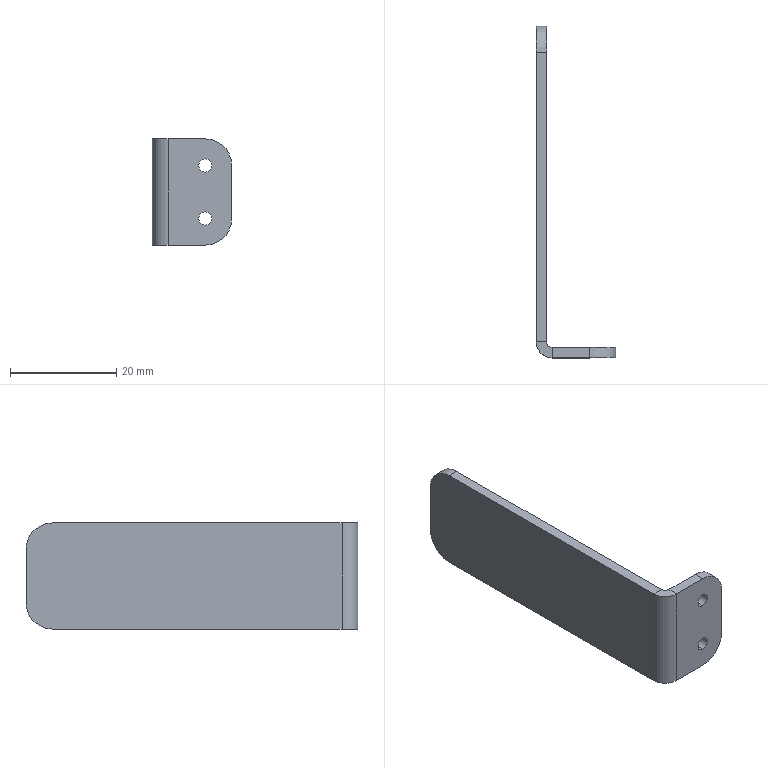Part | SolidWorks | features BreakCorner 1, FlatPattern 1, HoleWzd 1, SMBaseFlange 1, SheetMetal 1 | 1 solid | 22 faces | box 15 x 62.5 x 20 mm | volume 2923 mm3 | plane 12 | cylinder 10 | commonest cylinder face diameters 2.5 x4 10 x4 2 x1 6 x1
STEP:
#1=CARTESIAN_POINT('',(10.,0.,-6.25));
#2=VERTEX_POINT('',#1);
#3=CARTESIAN_POINT('',(10.,0.,-3.75));
#4=VERTEX_POINT('',#3);
#5=CARTESIAN_POINT('',(10.,0.,-5.));
#6=DIRECTION('',(0.,1.,0.));
#7=DIRECTION('',(0.,0.,1.));
#8=AXIS2_PLACEMENT_3D('',#5,#6,#7);
#9=CIRCLE('',#8,1.25);
#10=EDGE_CURVE('',#2,#4,#9,.T.);
#11=ORIENTED_EDGE('',*,*,#10,.F.);
#12=CARTESIAN_POINT('',(10.,2.,-6.25));
#13=VERTEX_POINT('',#12);
#14=CARTESIAN_POINT('',(10.,2.,-6.25));
#15=DIRECTION('',(0.,1.,0.));
#16=VECTOR('',#15,1000.);
#17=LINE('',#14,#16);
#18=EDGE_CURVE('',#2,#13,#17,.T.);
#19=ORIENTED_EDGE('',*,*,#18,.T.);
#20=CARTESIAN_POINT('',(10.,2.,-3.75));
#21=VERTEX_POINT('',#20);
#22=CARTESIAN_POINT('',(10.,2.,-5.));
#23=DIRECTION('',(0.,1.,0.));
#24=DIRECTION('',(0.,0.,1.));
#25=AXIS2_PLACEMENT_3D('',#22,#23,#24);
#26=CIRCLE('',#25,1.25);
#27=EDGE_CURVE('',#13,#21,#26,.T.);
#28=ORIENTED_EDGE('',*,*,#27,.T.);
#29=CARTESIAN_POINT('',(10.,2.,-3.75));
#30=DIRECTION('',(0.,1.,0.));
#31=VECTOR('',#30,1000.);
#32=LINE('',#29,#31);
#33=EDGE_CURVE('',#4,#21,#32,.T.);
#34=ORIENTED_EDGE('',*,*,#33,.F.);
#35=EDGE_LOOP('',(#11,#19,#28,#34));
#36=FACE_OUTER_BOUND('',#35,.T.);
#37=CARTESIAN_POINT('',(10.,2.,-5.));
#38=DIRECTION('',(0.,1.,0.));
#39=DIRECTION('',(0.,0.,1.));
#40=AXIS2_PLACEMENT_3D('',#37,#38,#39);
#41=CYLINDRICAL_SURFACE('',#40,1.25);
#42=ADVANCED_FACE('',(#36),#41,.F.);
#43=CARTESIAN_POINT('',(10.,0.,3.75));
#44=VERTEX_POINT('',#43);
#45=CARTESIAN_POINT('',(10.,0.,6.25));
#46=VERTEX_POINT('',#45);
#47=CARTESIAN_POINT('',(10.,0.,5.));
#48=DIRECTION('',(0.,1.,0.));
#49=DIRECTION('',(0.,0.,1.));
#50=AXIS2_PLACEMENT_3D('',#47,#48,#49);
#51=CIRCLE('',#50,1.25);
#52=EDGE_CURVE('',#44,#46,#51,.T.);
#53=ORIENTED_EDGE('',*,*,#52,.F.);
#54=CARTESIAN_POINT('',(10.,2.,3.75));
#55=VERTEX_POINT('',#54);
#56=CARTESIAN_POINT('',(10.,2.,3.75));
#57=DIRECTION('',(0.,1.,0.));
#58=VECTOR('',#57,1000.);
#59=LINE('',#56,#58);
#60=EDGE_CURVE('',#44,#55,#59,.T.);
#61=ORIENTED_EDGE('',*,*,#60,.T.);
#62=CARTESIAN_POINT('',(10.,2.,6.25));
#63=VERTEX_POINT('',#62);
#64=CARTESIAN_POINT('',(10.,2.,5.));
#65=DIRECTION('',(0.,1.,0.));
#66=DIRECTION('',(0.,0.,1.));
#67=AXIS2_PLACEMENT_3D('',#64,#65,#66);
#68=CIRCLE('',#67,1.25);
#69=EDGE_CURVE('',#55,#63,#68,.T.);
#70=ORIENTED_EDGE('',*,*,#69,.T.);
#71=CARTESIAN_POINT('',(10.,2.,6.25));
#72=DIRECTION('',(0.,1.,0.));
#73=VECTOR('',#72,1000.);
#74=LINE('',#71,#73);
#75=EDGE_CURVE('',#46,#63,#74,.T.);
#76=ORIENTED_EDGE('',*,*,#75,.F.);
#77=EDGE_LOOP('',(#53,#61,#70,#76));
#78=FACE_OUTER_BOUND('',#77,.T.);
#79=CARTESIAN_POINT('',(10.,2.,5.));
#80=DIRECTION('',(0.,1.,0.));
#81=DIRECTION('',(0.,0.,1.));
#82=AXIS2_PLACEMENT_3D('',#79,#80,#81);
#83=CYLINDRICAL_SURFACE('',#82,1.25);
#84=ADVANCED_FACE('',(#78),#83,.F.);
#85=CARTESIAN_POINT('',(0.,3.,10.));
#86=VERTEX_POINT('',#85);
#87=CARTESIAN_POINT('',(2.,3.,10.));
#88=VERTEX_POINT('',#87);
#89=CARTESIAN_POINT('',(0.,3.,10.));
#90=DIRECTION('',(1.,0.,0.));
#91=VECTOR('',#90,1000.);
#92=LINE('',#89,#91);
#93=EDGE_CURVE('',#86,#88,#92,.T.);
#94=ORIENTED_EDGE('',*,*,#93,.F.);
#95=CARTESIAN_POINT('',(3.,0.,10.));
#96=VERTEX_POINT('',#95);
#97=CARTESIAN_POINT('',(3.,3.,10.));
#98=DIRECTION('',(0.,0.,1.));
#99=DIRECTION('',(-1.,0.,0.));
#100=AXIS2_PLACEMENT_3D('',#97,#98,#99);
#101=CIRCLE('',#100,3.);
#102=EDGE_CURVE('',#86,#96,#101,.T.);
#103=ORIENTED_EDGE('',*,*,#102,.T.);
#104=CARTESIAN_POINT('',(3.,2.,10.));
#105=VERTEX_POINT('',#104);
#106=CARTESIAN_POINT('',(3.,2.,10.));
#107=DIRECTION('',(0.,-1.,0.));
#108=VECTOR('',#107,1000.);
#109=LINE('',#106,#108);
#110=EDGE_CURVE('',#105,#96,#109,.T.);
#111=ORIENTED_EDGE('',*,*,#110,.F.);
#112=CARTESIAN_POINT('',(3.,3.,10.));
#113=DIRECTION('',(0.,0.,1.));
#114=DIRECTION('',(1.,0.,0.));
#115=AXIS2_PLACEMENT_3D('',#112,#113,#114);
#116=CIRCLE('',#115,1.);
#117=EDGE_CURVE('',#88,#105,#116,.T.);
#118=ORIENTED_EDGE('',*,*,#117,.F.);
#119=EDGE_LOOP('',(#94,#103,#111,#118));
#120=FACE_OUTER_BOUND('',#119,.T.);
#121=CARTESIAN_POINT('',(0.,3.,10.));
#122=DIRECTION('',(0.,0.,1.));
#123=DIRECTION('',(1.,0.,0.));
#124=AXIS2_PLACEMENT_3D('',#121,#122,#123);
#125=PLANE('',#124);
#126=ADVANCED_FACE('',(#120),#125,.T.);
#127=CARTESIAN_POINT('',(2.,57.5,10.));
#128=VERTEX_POINT('',#127);
#129=CARTESIAN_POINT('',(2.,62.5,10.));
#130=DIRECTION('',(0.,-1.,0.));
#131=VECTOR('',#130,1000.);
#132=LINE('',#129,#131);
#133=EDGE_CURVE('',#128,#88,#132,.T.);
#134=ORIENTED_EDGE('',*,*,#133,.F.);
#135=CARTESIAN_POINT('',(0.,57.5,10.));
#136=VERTEX_POINT('',#135);
#137=CARTESIAN_POINT('',(3.,57.5,10.));
#138=DIRECTION('',(-1.,0.,0.));
#139=VECTOR('',#138,1000.);
#140=LINE('',#137,#139);
#141=EDGE_CURVE('',#128,#136,#140,.T.);
#142=ORIENTED_EDGE('',*,*,#141,.T.);
#143=CARTESIAN_POINT('',(0.,62.5,10.));
#144=DIRECTION('',(0.,-1.,0.));
#145=VECTOR('',#144,1000.);
#146=LINE('',#143,#145);
#147=EDGE_CURVE('',#136,#86,#146,.T.);
#148=ORIENTED_EDGE('',*,*,#147,.T.);
#149=ORIENTED_EDGE('',*,*,#93,.T.);
#150=EDGE_LOOP('',(#134,#142,#148,#149));
#151=FACE_OUTER_BOUND('',#150,.T.);
#152=CARTESIAN_POINT('',(3.,2.,10.));
#153=DIRECTION('',(0.,0.,1.));
#154=DIRECTION('',(1.,0.,0.));
#155=AXIS2_PLACEMENT_3D('',#152,#153,#154);
#156=PLANE('',#155);
#157=ADVANCED_FACE('',(#151),#156,.T.);
#158=CARTESIAN_POINT('',(3.,0.,-10.));
#159=VERTEX_POINT('',#158);
#160=CARTESIAN_POINT('',(3.,2.,-10.));
#161=VERTEX_POINT('',#160);
#162=CARTESIAN_POINT('',(3.,0.,-10.));
#163=DIRECTION('',(0.,1.,0.));
#164=VECTOR('',#163,1000.);
#165=LINE('',#162,#164);
#166=EDGE_CURVE('',#159,#161,#165,.T.);
#167=ORIENTED_EDGE('',*,*,#166,.F.);
#168=CARTESIAN_POINT('',(0.,3.,-10.));
#169=VERTEX_POINT('',#168);
#170=CARTESIAN_POINT('',(3.,3.,-10.));
#171=DIRECTION('',(0.,0.,1.));
#172=DIRECTION('',(-1.,0.,0.));
#173=AXIS2_PLACEMENT_3D('',#170,#171,#172);
#174=CIRCLE('',#173,3.);
#175=EDGE_CURVE('',#169,#159,#174,.T.);
#176=ORIENTED_EDGE('',*,*,#175,.F.);
#177=CARTESIAN_POINT('',(2.,3.,-10.));
#178=VERTEX_POINT('',#177);
#179=CARTESIAN_POINT('',(2.,3.,-10.));
#180=DIRECTION('',(-1.,0.,0.));
#181=VECTOR('',#180,1000.);
#182=LINE('',#179,#181);
#183=EDGE_CURVE('',#178,#169,#182,.T.);
#184=ORIENTED_EDGE('',*,*,#183,.F.);
#185=CARTESIAN_POINT('',(3.,3.,-10.));
#186=DIRECTION('',(0.,0.,1.));
#187=DIRECTION('',(1.,0.,0.));
#188=AXIS2_PLACEMENT_3D('',#185,#186,#187);
#189=CIRCLE('',#188,1.);
#190=EDGE_CURVE('',#178,#161,#189,.T.);
#191=ORIENTED_EDGE('',*,*,#190,.T.);
#192=EDGE_LOOP('',(#167,#176,#184,#191));
#193=FACE_OUTER_BOUND('',#192,.T.);
#194=CARTESIAN_POINT('',(3.,0.,-10.));
#195=DIRECTION('',(0.,0.,-1.));
#196=DIRECTION('',(-1.,0.,0.));
#197=AXIS2_PLACEMENT_3D('',#194,#195,#196);
#198=PLANE('',#197);
#199=ADVANCED_FACE('',(#193),#198,.T.);
#200=CARTESIAN_POINT('',(10.,2.,-10.));
#201=VERTEX_POINT('',#200);
#202=CARTESIAN_POINT('',(0.,2.,-10.));
#203=DIRECTION('',(1.,0.,0.));
#204=VECTOR('',#203,1000.);
#205=LINE('',#202,#204);
#206=EDGE_CURVE('',#161,#201,#205,.T.);
#207=ORIENTED_EDGE('',*,*,#206,.T.);
#208=CARTESIAN_POINT('',(10.,0.,-10.));
#209=VERTEX_POINT('',#208);
#210=CARTESIAN_POINT('',(10.,3.,-10.));
#211=DIRECTION('',(0.,-1.,0.));
#212=VECTOR('',#211,1000.);
#213=LINE('',#210,#212);
#214=EDGE_CURVE('',#201,#209,#213,.T.);
#215=ORIENTED_EDGE('',*,*,#214,.T.);
#216=CARTESIAN_POINT('',(0.,0.,-10.));
#217=DIRECTION('',(1.,0.,0.));
#218=VECTOR('',#217,1000.);
#219=LINE('',#216,#218);
#220=EDGE_CURVE('',#159,#209,#219,.T.);
#221=ORIENTED_EDGE('',*,*,#220,.F.);
#222=ORIENTED_EDGE('',*,*,#166,.T.);
#223=EDGE_LOOP('',(#207,#215,#221,#222));
#224=FACE_OUTER_BOUND('',#223,.T.);
#225=CARTESIAN_POINT('',(2.,3.,-10.));
#226=DIRECTION('',(0.,0.,-1.));
#227=DIRECTION('',(-1.,0.,0.));
#228=AXIS2_PLACEMENT_3D('',#225,#226,#227);
#229=PLANE('',#228);
#230=ADVANCED_FACE('',(#224),#229,.T.);
#231=CARTESIAN_POINT('',(10.,0.,-5.));
#232=DIRECTION('',(0.,1.,0.));
#233=DIRECTION('',(0.,0.,1.));
#234=AXIS2_PLACEMENT_3D('',#231,#232,#233);
#235=CIRCLE('',#234,1.25);
#236=EDGE_CURVE('',#4,#2,#235,.T.);
#237=ORIENTED_EDGE('',*,*,#236,.T.);
#238=ORIENTED_EDGE('',*,*,#10,.T.);
#239=EDGE_LOOP('',(#237,#238));
#240=FACE_BOUND('',#239,.T.);
#241=CARTESIAN_POINT('',(10.,0.,5.));
#242=DIRECTION('',(0.,1.,0.));
#243=DIRECTION('',(0.,0.,1.));
#244=AXIS2_PLACEMENT_3D('',#241,#242,#243);
#245=CIRCLE('',#244,1.25);
#246=EDGE_CURVE('',#46,#44,#245,.T.);
#247=ORIENTED_EDGE('',*,*,#246,.T.);
#248=ORIENTED_EDGE('',*,*,#52,.T.);
#249=EDGE_LOOP('',(#247,#248));
#250=FACE_BOUND('',#249,.T.);
#251=CARTESIAN_POINT('',(15.,0.,5.));
#252=VERTEX_POINT('',#251);
#253=CARTESIAN_POINT('',(15.,0.,-5.));
#254=VERTEX_POINT('',#253);
#255=CARTESIAN_POINT('',(15.,0.,10.));
#256=DIRECTION('',(0.,0.,-1.));
#257=VECTOR('',#256,1000.);
#258=LINE('',#255,#257);
#259=EDGE_CURVE('',#252,#254,#258,.T.);
#260=ORIENTED_EDGE('',*,*,#259,.F.);
#261=CARTESIAN_POINT('',(10.,0.,10.));
#262=VERTEX_POINT('',#261);
#263=CARTESIAN_POINT('',(10.,0.,5.));
#264=DIRECTION('',(0.,-1.,0.));
#265=DIRECTION('',(0.,0.,1.));
#266=AXIS2_PLACEMENT_3D('',#263,#264,#265);
#267=CIRCLE('',#266,5.);
#268=EDGE_CURVE('',#252,#262,#267,.T.);
#269=ORIENTED_EDGE('',*,*,#268,.T.);
#270=CARTESIAN_POINT('',(0.,0.,10.));
#271=DIRECTION('',(1.,0.,0.));
#272=VECTOR('',#271,1000.);
#273=LINE('',#270,#272);
#274=EDGE_CURVE('',#96,#262,#273,.T.);
#275=ORIENTED_EDGE('',*,*,#274,.F.);
#276=CARTESIAN_POINT('',(3.,0.,10.));
#277=DIRECTION('',(0.,0.,-1.));
#278=VECTOR('',#277,1000.);
#279=LINE('',#276,#278);
#280=EDGE_CURVE('',#96,#159,#279,.T.);
#281=ORIENTED_EDGE('',*,*,#280,.T.);
#282=ORIENTED_EDGE('',*,*,#220,.T.);
#283=CARTESIAN_POINT('',(10.,0.,-5.));
#284=DIRECTION('',(0.,-1.,0.));
#285=DIRECTION('',(0.,0.,1.));
#286=AXIS2_PLACEMENT_3D('',#283,#284,#285);
#287=CIRCLE('',#286,5.);
#288=EDGE_CURVE('',#209,#254,#287,.T.);
#289=ORIENTED_EDGE('',*,*,#288,.T.);
#290=EDGE_LOOP('',(#260,#269,#275,#281,#282,#289));
#291=FACE_OUTER_BOUND('',#290,.T.);
#292=CARTESIAN_POINT('',(0.,0.,10.));
#293=DIRECTION('',(0.,1.,0.));
#294=DIRECTION('',(0.,0.,1.));
#295=AXIS2_PLACEMENT_3D('',#292,#293,#294);
#296=PLANE('',#295);
#297=ADVANCED_FACE('',(#240,#250,#291),#296,.F.);
#298=CARTESIAN_POINT('',(15.,2.,5.));
#299=VERTEX_POINT('',#298);
#300=CARTESIAN_POINT('',(15.,2.,-5.));
#301=VERTEX_POINT('',#300);
#302=CARTESIAN_POINT('',(15.,2.,10.));
#303=DIRECTION('',(0.,0.,-1.));
#304=VECTOR('',#303,1000.);
#305=LINE('',#302,#304);
#306=EDGE_CURVE('',#299,#301,#305,.T.);
#307=ORIENTED_EDGE('',*,*,#306,.F.);
#308=CARTESIAN_POINT('',(15.,2.,5.));
#309=DIRECTION('',(0.,-1.,0.));
#310=VECTOR('',#309,1000.);
#311=LINE('',#308,#310);
#312=EDGE_CURVE('',#299,#252,#311,.T.);
#313=ORIENTED_EDGE('',*,*,#312,.T.);
#314=ORIENTED_EDGE('',*,*,#259,.T.);
#315=CARTESIAN_POINT('',(15.,2.,-5.));
#316=DIRECTION('',(0.,1.,0.));
#317=VECTOR('',#316,1000.);
#318=LINE('',#315,#317);
#319=EDGE_CURVE('',#254,#301,#318,.T.);
#320=ORIENTED_EDGE('',*,*,#319,.T.);
#321=EDGE_LOOP('',(#307,#313,#314,#320));
#322=FACE_OUTER_BOUND('',#321,.T.);
#323=CARTESIAN_POINT('',(15.,2.,10.));
#324=DIRECTION('',(1.,0.,0.));
#325=DIRECTION('',(0.,0.,-1.));
#326=AXIS2_PLACEMENT_3D('',#323,#324,#325);
#327=PLANE('',#326);
#328=ADVANCED_FACE('',(#322),#327,.T.);
#329=CARTESIAN_POINT('',(10.,2.,-5.));
#330=DIRECTION('',(0.,1.,0.));
#331=DIRECTION('',(0.,0.,1.));
#332=AXIS2_PLACEMENT_3D('',#329,#330,#331);
#333=CIRCLE('',#332,1.25);
#334=EDGE_CURVE('',#21,#13,#333,.T.);
#335=ORIENTED_EDGE('',*,*,#334,.F.);
#336=ORIENTED_EDGE('',*,*,#27,.F.);
#337=EDGE_LOOP('',(#335,#336));
#338=FACE_BOUND('',#337,.T.);
#339=CARTESIAN_POINT('',(10.,2.,5.));
#340=DIRECTION('',(0.,1.,0.));
#341=DIRECTION('',(0.,0.,1.));
#342=AXIS2_PLACEMENT_3D('',#339,#340,#341);
#343=CIRCLE('',#342,1.25);
#344=EDGE_CURVE('',#63,#55,#343,.T.);
#345=ORIENTED_EDGE('',*,*,#344,.F.);
#346=ORIENTED_EDGE('',*,*,#69,.F.);
#347=EDGE_LOOP('',(#345,#346));
#348=FACE_BOUND('',#347,.T.);
#349=CARTESIAN_POINT('',(10.,2.,10.));
#350=VERTEX_POINT('',#349);
#351=CARTESIAN_POINT('',(0.,2.,10.));
#352=DIRECTION('',(1.,0.,0.));
#353=VECTOR('',#352,1000.);
#354=LINE('',#351,#353);
#355=EDGE_CURVE('',#105,#350,#354,.T.);
#356=ORIENTED_EDGE('',*,*,#355,.T.);
#357=CARTESIAN_POINT('',(10.,2.,5.));
#358=DIRECTION('',(0.,1.,0.));
#359=DIRECTION('',(0.,0.,1.));
#360=AXIS2_PLACEMENT_3D('',#357,#358,#359);
#361=CIRCLE('',#360,5.);
#362=EDGE_CURVE('',#350,#299,#361,.T.);
#363=ORIENTED_EDGE('',*,*,#362,.T.);
#364=ORIENTED_EDGE('',*,*,#306,.T.);
#365=CARTESIAN_POINT('',(10.,2.,-5.));
#366=DIRECTION('',(0.,1.,0.));
#367=DIRECTION('',(0.,0.,1.));
#368=AXIS2_PLACEMENT_3D('',#365,#366,#367);
#369=CIRCLE('',#368,5.);
#370=EDGE_CURVE('',#301,#201,#369,.T.);
#371=ORIENTED_EDGE('',*,*,#370,.T.);
#372=ORIENTED_EDGE('',*,*,#206,.F.);
#373=CARTESIAN_POINT('',(3.,2.,10.));
#374=DIRECTION('',(0.,0.,-1.));
#375=VECTOR('',#374,1000.);
#376=LINE('',#373,#375);
#377=EDGE_CURVE('',#105,#161,#376,.T.);
#378=ORIENTED_EDGE('',*,*,#377,.F.);
#379=EDGE_LOOP('',(#356,#363,#364,#371,#372,#378));
#380=FACE_OUTER_BOUND('',#379,.T.);
#381=CARTESIAN_POINT('',(0.,2.,10.));
#382=DIRECTION('',(0.,1.,0.));
#383=DIRECTION('',(0.,0.,1.));
#384=AXIS2_PLACEMENT_3D('',#381,#382,#383);
#385=PLANE('',#384);
#386=ADVANCED_FACE('',(#338,#348,#380),#385,.T.);
#387=ORIENTED_EDGE('',*,*,#190,.F.);
#388=CARTESIAN_POINT('',(2.,3.,10.));
#389=DIRECTION('',(0.,0.,-1.));
#390=VECTOR('',#389,1000.);
#391=LINE('',#388,#390);
#392=EDGE_CURVE('',#88,#178,#391,.T.);
#393=ORIENTED_EDGE('',*,*,#392,.F.);
#394=ORIENTED_EDGE('',*,*,#117,.T.);
#395=ORIENTED_EDGE('',*,*,#377,.T.);
#396=EDGE_LOOP('',(#387,#393,#394,#395));
#397=FACE_OUTER_BOUND('',#396,.T.);
#398=CARTESIAN_POINT('',(3.,3.,10.));
#399=DIRECTION('',(0.,0.,-1.));
#400=DIRECTION('',(-1.,0.,0.));
#401=AXIS2_PLACEMENT_3D('',#398,#399,#400);
#402=CYLINDRICAL_SURFACE('',#401,1.);
#403=ADVANCED_FACE('',(#397),#402,.F.);
#404=CARTESIAN_POINT('',(2.,62.5,5.));
#405=VERTEX_POINT('',#404);
#406=CARTESIAN_POINT('',(2.,62.5,-5.));
#407=VERTEX_POINT('',#406);
#408=CARTESIAN_POINT('',(2.,62.5,10.));
#409=DIRECTION('',(0.,0.,-1.));
#410=VECTOR('',#409,1000.);
#411=LINE('',#408,#410);
#412=EDGE_CURVE('',#405,#407,#411,.T.);
#413=ORIENTED_EDGE('',*,*,#412,.F.);
#414=CARTESIAN_POINT('',(2.,57.5,5.));
#415=DIRECTION('',(1.,0.,0.));
#416=DIRECTION('',(0.,1.,0.));
#417=AXIS2_PLACEMENT_3D('',#414,#415,#416);
#418=CIRCLE('',#417,5.);
#419=EDGE_CURVE('',#405,#128,#418,.T.);
#420=ORIENTED_EDGE('',*,*,#419,.T.);
#421=ORIENTED_EDGE('',*,*,#133,.T.);
#422=ORIENTED_EDGE('',*,*,#392,.T.);
#423=CARTESIAN_POINT('',(2.,57.5,-10.));
#424=VERTEX_POINT('',#423);
#425=CARTESIAN_POINT('',(2.,62.5,-10.));
#426=DIRECTION('',(0.,-1.,0.));
#427=VECTOR('',#426,1000.);
#428=LINE('',#425,#427);
#429=EDGE_CURVE('',#424,#178,#428,.T.);
#430=ORIENTED_EDGE('',*,*,#429,.F.);
#431=CARTESIAN_POINT('',(2.,57.5,-5.));
#432=DIRECTION('',(1.,0.,0.));
#433=DIRECTION('',(0.,1.,0.));
#434=AXIS2_PLACEMENT_3D('',#431,#432,#433);
#435=CIRCLE('',#434,5.);
#436=EDGE_CURVE('',#424,#407,#435,.T.);
#437=ORIENTED_EDGE('',*,*,#436,.T.);
#438=EDGE_LOOP('',(#413,#420,#421,#422,#430,#437));
#439=FACE_OUTER_BOUND('',#438,.T.);
#440=CARTESIAN_POINT('',(2.,62.5,10.));
#441=DIRECTION('',(1.,0.,0.));
#442=DIRECTION('',(0.,1.,0.));
#443=AXIS2_PLACEMENT_3D('',#440,#441,#442);
#444=PLANE('',#443);
#445=ADVANCED_FACE('',(#439),#444,.T.);
#446=CARTESIAN_POINT('',(0.,62.5,5.));
#447=VERTEX_POINT('',#446);
#448=CARTESIAN_POINT('',(0.,62.5,-5.));
#449=VERTEX_POINT('',#448);
#450=CARTESIAN_POINT('',(0.,62.5,10.));
#451=DIRECTION('',(0.,0.,-1.));
#452=VECTOR('',#451,1000.);
#453=LINE('',#450,#452);
#454=EDGE_CURVE('',#447,#449,#453,.T.);
#455=ORIENTED_EDGE('',*,*,#454,.F.);
#456=CARTESIAN_POINT('',(0.,62.5,5.));
#457=DIRECTION('',(1.,0.,0.));
#458=VECTOR('',#457,1000.);
#459=LINE('',#456,#458);
#460=EDGE_CURVE('',#447,#405,#459,.T.);
#461=ORIENTED_EDGE('',*,*,#460,.T.);
#462=ORIENTED_EDGE('',*,*,#412,.T.);
#463=CARTESIAN_POINT('',(0.,62.5,-5.));
#464=DIRECTION('',(-1.,0.,0.));
#465=VECTOR('',#464,1000.);
#466=LINE('',#463,#465);
#467=EDGE_CURVE('',#407,#449,#466,.T.);
#468=ORIENTED_EDGE('',*,*,#467,.T.);
#469=EDGE_LOOP('',(#455,#461,#462,#468));
#470=FACE_OUTER_BOUND('',#469,.T.);
#471=CARTESIAN_POINT('',(0.,62.5,10.));
#472=DIRECTION('',(0.,1.,0.));
#473=DIRECTION('',(0.,0.,1.));
#474=AXIS2_PLACEMENT_3D('',#471,#472,#473);
#475=PLANE('',#474);
#476=ADVANCED_FACE('',(#470),#475,.T.);
#477=ORIENTED_EDGE('',*,*,#147,.F.);
#478=CARTESIAN_POINT('',(0.,57.5,5.));
#479=DIRECTION('',(-1.,0.,0.));
#480=DIRECTION('',(0.,1.,0.));
#481=AXIS2_PLACEMENT_3D('',#478,#479,#480);
#482=CIRCLE('',#481,5.);
#483=EDGE_CURVE('',#136,#447,#482,.T.);
#484=ORIENTED_EDGE('',*,*,#483,.T.);
#485=ORIENTED_EDGE('',*,*,#454,.T.);
#486=CARTESIAN_POINT('',(0.,57.5,-10.));
#487=VERTEX_POINT('',#486);
#488=CARTESIAN_POINT('',(0.,57.5,-5.));
#489=DIRECTION('',(-1.,0.,0.));
#490=DIRECTION('',(0.,1.,0.));
#491=AXIS2_PLACEMENT_3D('',#488,#489,#490);
#492=CIRCLE('',#491,5.);
#493=EDGE_CURVE('',#449,#487,#492,.T.);
#494=ORIENTED_EDGE('',*,*,#493,.T.);
#495=CARTESIAN_POINT('',(0.,62.5,-10.));
#496=DIRECTION('',(0.,-1.,0.));
#497=VECTOR('',#496,1000.);
#498=LINE('',#495,#497);
#499=EDGE_CURVE('',#487,#169,#498,.T.);
#500=ORIENTED_EDGE('',*,*,#499,.T.);
#501=CARTESIAN_POINT('',(0.,3.,10.));
#502=DIRECTION('',(0.,0.,-1.));
#503=VECTOR('',#502,1000.);
#504=LINE('',#501,#503);
#505=EDGE_CURVE('',#86,#169,#504,.T.);
#506=ORIENTED_EDGE('',*,*,#505,.F.);
#507=EDGE_LOOP('',(#477,#484,#485,#494,#500,#506));
#508=FACE_OUTER_BOUND('',#507,.T.);
#509=CARTESIAN_POINT('',(0.,62.5,10.));
#510=DIRECTION('',(1.,0.,0.));
#511=DIRECTION('',(0.,1.,0.));
#512=AXIS2_PLACEMENT_3D('',#509,#510,#511);
#513=PLANE('',#512);
#514=ADVANCED_FACE('',(#508),#513,.F.);
#515=ORIENTED_EDGE('',*,*,#175,.T.);
#516=ORIENTED_EDGE('',*,*,#280,.F.);
#517=ORIENTED_EDGE('',*,*,#102,.F.);
#518=ORIENTED_EDGE('',*,*,#505,.T.);
#519=EDGE_LOOP('',(#515,#516,#517,#518));
#520=FACE_OUTER_BOUND('',#519,.T.);
#521=CARTESIAN_POINT('',(3.,3.,10.));
#522=DIRECTION('',(0.,0.,-1.));
#523=DIRECTION('',(-1.,0.,0.));
#524=AXIS2_PLACEMENT_3D('',#521,#522,#523);
#525=CYLINDRICAL_SURFACE('',#524,3.);
#526=ADVANCED_FACE('',(#520),#525,.T.);
#527=ORIENTED_EDGE('',*,*,#274,.T.);
#528=CARTESIAN_POINT('',(10.,3.,10.));
#529=DIRECTION('',(0.,1.,0.));
#530=VECTOR('',#529,1000.);
#531=LINE('',#528,#530);
#532=EDGE_CURVE('',#262,#350,#531,.T.);
#533=ORIENTED_EDGE('',*,*,#532,.T.);
#534=ORIENTED_EDGE('',*,*,#355,.F.);
#535=ORIENTED_EDGE('',*,*,#110,.T.);
#536=EDGE_LOOP('',(#527,#533,#534,#535));
#537=FACE_OUTER_BOUND('',#536,.T.);
#538=CARTESIAN_POINT('',(3.,3.,10.));
#539=DIRECTION('',(0.,0.,1.));
#540=DIRECTION('',(1.,0.,0.));
#541=AXIS2_PLACEMENT_3D('',#538,#539,#540);
#542=PLANE('',#541);
#543=ADVANCED_FACE('',(#537),#542,.T.);
#544=ORIENTED_EDGE('',*,*,#499,.F.);
#545=CARTESIAN_POINT('',(2.,57.5,-10.));
#546=DIRECTION('',(1.,0.,0.));
#547=VECTOR('',#546,1000.);
#548=LINE('',#545,#547);
#549=EDGE_CURVE('',#487,#424,#548,.T.);
#550=ORIENTED_EDGE('',*,*,#549,.T.);
#551=ORIENTED_EDGE('',*,*,#429,.T.);
#552=ORIENTED_EDGE('',*,*,#183,.T.);
#553=EDGE_LOOP('',(#544,#550,#551,#552));
#554=FACE_OUTER_BOUND('',#553,.T.);
#555=CARTESIAN_POINT('',(3.,3.,-10.));
#556=DIRECTION('',(0.,0.,1.));
#557=DIRECTION('',(1.,0.,0.));
#558=AXIS2_PLACEMENT_3D('',#555,#556,#557);
#559=PLANE('',#558);
#560=ADVANCED_FACE('',(#554),#559,.F.);
#561=ORIENTED_EDGE('',*,*,#483,.F.);
#562=ORIENTED_EDGE('',*,*,#141,.F.);
#563=ORIENTED_EDGE('',*,*,#419,.F.);
#564=ORIENTED_EDGE('',*,*,#460,.F.);
#565=EDGE_LOOP('',(#561,#562,#563,#564));
#566=FACE_OUTER_BOUND('',#565,.T.);
#567=CARTESIAN_POINT('',(0.,57.5,5.));
#568=DIRECTION('',(1.,0.,0.));
#569=DIRECTION('',(0.,0.,-1.));
#570=AXIS2_PLACEMENT_3D('',#567,#568,#569);
#571=CYLINDRICAL_SURFACE('',#570,5.);
#572=ADVANCED_FACE('',(#566),#571,.T.);
#573=ORIENTED_EDGE('',*,*,#493,.F.);
#574=ORIENTED_EDGE('',*,*,#467,.F.);
#575=ORIENTED_EDGE('',*,*,#436,.F.);
#576=ORIENTED_EDGE('',*,*,#549,.F.);
#577=EDGE_LOOP('',(#573,#574,#575,#576));
#578=FACE_OUTER_BOUND('',#577,.T.);
#579=CARTESIAN_POINT('',(3.,57.5,-5.));
#580=DIRECTION('',(-1.,0.,0.));
#581=DIRECTION('',(0.,0.,1.));
#582=AXIS2_PLACEMENT_3D('',#579,#580,#581);
#583=CYLINDRICAL_SURFACE('',#582,5.);
#584=ADVANCED_FACE('',(#578),#583,.T.);
#585=ORIENTED_EDGE('',*,*,#362,.F.);
#586=ORIENTED_EDGE('',*,*,#532,.F.);
#587=ORIENTED_EDGE('',*,*,#268,.F.);
#588=ORIENTED_EDGE('',*,*,#312,.F.);
#589=EDGE_LOOP('',(#585,#586,#587,#588));
#590=FACE_OUTER_BOUND('',#589,.T.);
#591=CARTESIAN_POINT('',(10.,2.,5.));
#592=DIRECTION('',(0.,-1.,0.));
#593=DIRECTION('',(0.,0.,-1.));
#594=AXIS2_PLACEMENT_3D('',#591,#592,#593);
#595=CYLINDRICAL_SURFACE('',#594,5.);
#596=ADVANCED_FACE('',(#590),#595,.T.);
#597=ORIENTED_EDGE('',*,*,#370,.F.);
#598=ORIENTED_EDGE('',*,*,#319,.F.);
#599=ORIENTED_EDGE('',*,*,#288,.F.);
#600=ORIENTED_EDGE('',*,*,#214,.F.);
#601=EDGE_LOOP('',(#597,#598,#599,#600));
#602=FACE_OUTER_BOUND('',#601,.T.);
#603=CARTESIAN_POINT('',(10.,3.,-5.));
#604=DIRECTION('',(0.,-1.,0.));
#605=DIRECTION('',(0.,0.,-1.));
#606=AXIS2_PLACEMENT_3D('',#603,#604,#605);
#607=CYLINDRICAL_SURFACE('',#606,5.);
#608=ADVANCED_FACE('',(#602),#607,.T.);
#609=ORIENTED_EDGE('',*,*,#60,.F.);
#610=ORIENTED_EDGE('',*,*,#246,.F.);
#611=ORIENTED_EDGE('',*,*,#75,.T.);
#612=ORIENTED_EDGE('',*,*,#344,.T.);
#613=EDGE_LOOP('',(#609,#610,#611,#612));
#614=FACE_OUTER_BOUND('',#613,.T.);
#615=CARTESIAN_POINT('',(10.,2.,5.));
#616=DIRECTION('',(0.,1.,0.));
#617=DIRECTION('',(0.,0.,1.));
#618=AXIS2_PLACEMENT_3D('',#615,#616,#617);
#619=CYLINDRICAL_SURFACE('',#618,1.25);
#620=ADVANCED_FACE('',(#614),#619,.F.);
#621=ORIENTED_EDGE('',*,*,#18,.F.);
#622=ORIENTED_EDGE('',*,*,#236,.F.);
#623=ORIENTED_EDGE('',*,*,#33,.T.);
#624=ORIENTED_EDGE('',*,*,#334,.T.);
#625=EDGE_LOOP('',(#621,#622,#623,#624));
#626=FACE_OUTER_BOUND('',#625,.T.);
#627=CARTESIAN_POINT('',(10.,2.,-5.));
#628=DIRECTION('',(0.,1.,0.));
#629=DIRECTION('',(0.,0.,1.));
#630=AXIS2_PLACEMENT_3D('',#627,#628,#629);
#631=CYLINDRICAL_SURFACE('',#630,1.25);
#632=ADVANCED_FACE('',(#626),#631,.F.);
#633=CLOSED_SHELL('',(#42,#84,#126,#157,#199,#230,#297,#328,#386,#403,#445,#476,#514,#526,#543,#560,#572,#584,#596,#608,#620,#632));
#634=MANIFOLD_SOLID_BREP('',#633);
#635=CARTESIAN_POINT('',(0.,0.,0.));
#636=DIRECTION('',(0.,0.,1.));
#637=DIRECTION('',(1.,0.,0.));
#638=AXIS2_PLACEMENT_3D('',#635,#636,#637);
#639=(LENGTH_UNIT()NAMED_UNIT(*)SI_UNIT(.MILLI.,.METRE.));
#640=UNCERTAINTY_MEASURE_WITH_UNIT(LENGTH_MEASURE(0.00001),#639,'','');
#641=(NAMED_UNIT(*)PLANE_ANGLE_UNIT()SI_UNIT($,.RADIAN.));
#642=(NAMED_UNIT(*)SI_UNIT($,.STERADIAN.)SOLID_ANGLE_UNIT());
#643=(GEOMETRIC_REPRESENTATION_CONTEXT(3)GLOBAL_UNCERTAINTY_ASSIGNED_CONTEXT((#640))GLOBAL_UNIT_ASSIGNED_CONTEXT((#639,#641,#642))REPRESENTATION_CONTEXT('',''));
#644=ADVANCED_BREP_SHAPE_REPRESENTATION('',(#634,#638),#643);